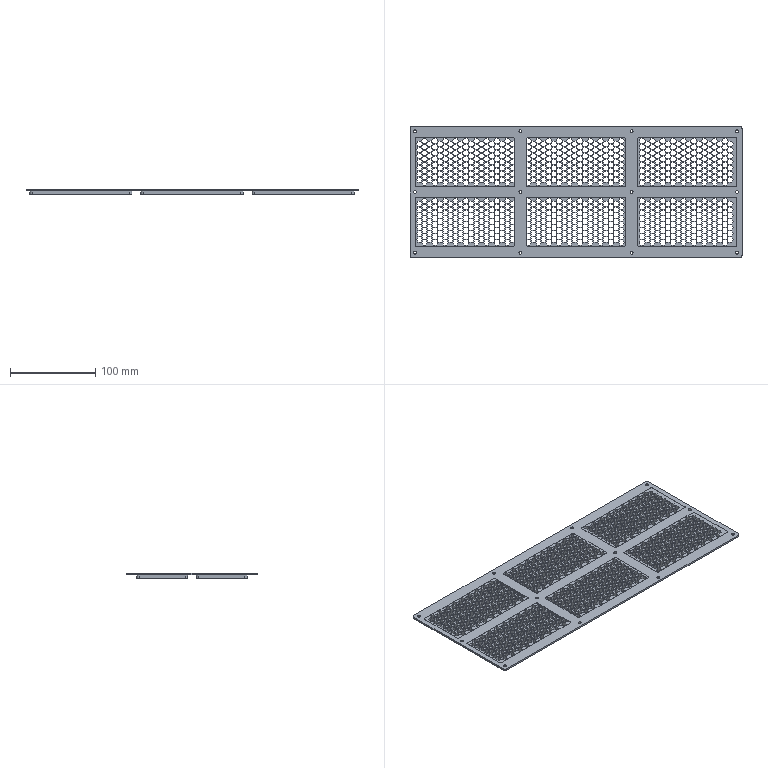Part | 1 solid | 5230 faces | volume 138364 mm3 | plane 5132 | cylinder 98 | commonest cylinder face diameters 2.5 x46 5.5 x28 3.5 x24